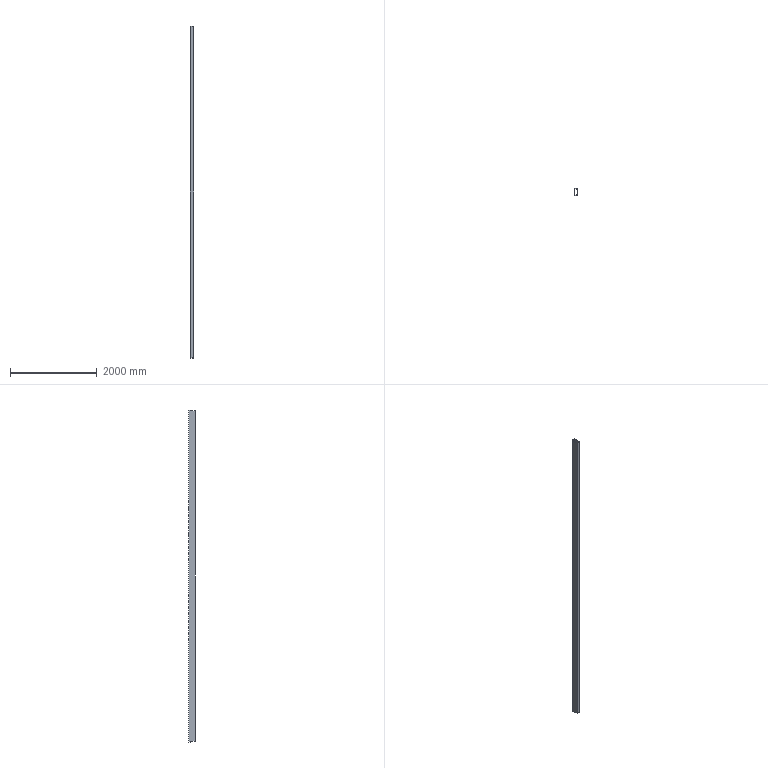Part | STEP file | 750078111 | 1 solid | 24 faces | box 80 x 160 x 7672 mm | volume 17309604 mm3 | plane 16 | cylinder 8 | commonest cylinder face diameters 4 x4 14 x4
STEP:
#1=CARTESIAN_POINT('',(-35.,-73.,3822.));
#2=VERTEX_POINT('',#1);
#3=CARTESIAN_POINT('',(-35.,28.5,3822.));
#4=VERTEX_POINT('',#3);
#5=CARTESIAN_POINT('',(-35.,-73.,3822.));
#6=DIRECTION('',(0.,1.,0.));
#7=VECTOR('',#6,1000.);
#8=LINE('',#5,#7);
#9=EDGE_CURVE('',#2,#4,#8,.T.);
#10=ORIENTED_EDGE('',*,*,#9,.F.);
#11=CARTESIAN_POINT('',(-35.,-73.,-3822.));
#12=VERTEX_POINT('',#11);
#13=CARTESIAN_POINT('',(-35.,-73.,3836.));
#14=DIRECTION('',(0.,0.,1.));
#15=VECTOR('',#14,1000.);
#16=LINE('',#13,#15);
#17=EDGE_CURVE('',#12,#2,#16,.T.);
#18=ORIENTED_EDGE('',*,*,#17,.F.);
#19=CARTESIAN_POINT('',(-35.,28.5,-3822.));
#20=VERTEX_POINT('',#19);
#21=CARTESIAN_POINT('',(-35.,-73.,-3822.));
#22=DIRECTION('',(0.,-1.,0.));
#23=VECTOR('',#22,1000.);
#24=LINE('',#21,#23);
#25=EDGE_CURVE('',#20,#12,#24,.T.);
#26=ORIENTED_EDGE('',*,*,#25,.F.);
#27=CARTESIAN_POINT('',(-35.,28.5,-3836.));
#28=VERTEX_POINT('',#27);
#29=CARTESIAN_POINT('',(-35.,28.5,3836.));
#30=DIRECTION('',(0.,0.,1.));
#31=VECTOR('',#30,1000.);
#32=LINE('',#29,#31);
#33=EDGE_CURVE('',#28,#20,#32,.T.);
#34=ORIENTED_EDGE('',*,*,#33,.F.);
#35=CARTESIAN_POINT('',(-35.,73.,-3836.));
#36=VERTEX_POINT('',#35);
#37=CARTESIAN_POINT('',(-35.,-73.,-3836.));
#38=DIRECTION('',(0.,-1.,0.));
#39=VECTOR('',#38,1000.);
#40=LINE('',#37,#39);
#41=EDGE_CURVE('',#36,#28,#40,.T.);
#42=ORIENTED_EDGE('',*,*,#41,.F.);
#43=CARTESIAN_POINT('',(-35.,73.,3836.));
#44=VERTEX_POINT('',#43);
#45=CARTESIAN_POINT('',(-35.,73.,3836.));
#46=DIRECTION('',(0.,0.,-1.));
#47=VECTOR('',#46,1000.);
#48=LINE('',#45,#47);
#49=EDGE_CURVE('',#44,#36,#48,.T.);
#50=ORIENTED_EDGE('',*,*,#49,.F.);
#51=CARTESIAN_POINT('',(-35.,28.5,3836.));
#52=VERTEX_POINT('',#51);
#53=CARTESIAN_POINT('',(-35.,-73.,3836.));
#54=DIRECTION('',(0.,1.,0.));
#55=VECTOR('',#54,1000.);
#56=LINE('',#53,#55);
#57=EDGE_CURVE('',#52,#44,#56,.T.);
#58=ORIENTED_EDGE('',*,*,#57,.F.);
#59=CARTESIAN_POINT('',(-35.,28.5,3836.));
#60=DIRECTION('',(0.,0.,1.));
#61=VECTOR('',#60,1000.);
#62=LINE('',#59,#61);
#63=EDGE_CURVE('',#4,#52,#62,.T.);
#64=ORIENTED_EDGE('',*,*,#63,.F.);
#65=EDGE_LOOP('',(#10,#18,#26,#34,#42,#50,#58,#64));
#66=FACE_OUTER_BOUND('',#65,.T.);
#67=CARTESIAN_POINT('',(-35.,-73.,3836.));
#68=DIRECTION('',(-1.,0.,0.));
#69=DIRECTION('',(0.,-1.,0.));
#70=AXIS2_PLACEMENT_3D('',#67,#68,#69);
#71=PLANE('',#70);
#72=ADVANCED_FACE('',(#66),#71,.F.);
#73=CARTESIAN_POINT('',(-40.,28.5,3822.));
#74=VERTEX_POINT('',#73);
#75=CARTESIAN_POINT('',(-40.,28.5,3836.));
#76=VERTEX_POINT('',#75);
#77=CARTESIAN_POINT('',(-40.,28.5,3822.));
#78=DIRECTION('',(0.,0.,1.));
#79=VECTOR('',#78,1000.);
#80=LINE('',#77,#79);
#81=EDGE_CURVE('',#74,#76,#80,.T.);
#82=ORIENTED_EDGE('',*,*,#81,.F.);
#83=CARTESIAN_POINT('',(-48.,28.5,3822.));
#84=DIRECTION('',(-1.,0.,0.));
#85=VECTOR('',#84,1000.);
#86=LINE('',#83,#85);
#87=EDGE_CURVE('',#4,#74,#86,.T.);
#88=ORIENTED_EDGE('',*,*,#87,.F.);
#89=ORIENTED_EDGE('',*,*,#63,.T.);
#90=CARTESIAN_POINT('',(-48.,28.5,3836.));
#91=DIRECTION('',(1.,0.,0.));
#92=VECTOR('',#91,1000.);
#93=LINE('',#90,#92);
#94=EDGE_CURVE('',#76,#52,#93,.T.);
#95=ORIENTED_EDGE('',*,*,#94,.F.);
#96=EDGE_LOOP('',(#82,#88,#89,#95));
#97=FACE_OUTER_BOUND('',#96,.T.);
#98=CARTESIAN_POINT('',(-48.,28.5,3822.));
#99=DIRECTION('',(0.,1.,0.));
#100=DIRECTION('',(-1.,0.,0.));
#101=AXIS2_PLACEMENT_3D('',#98,#99,#100);
#102=PLANE('',#101);
#103=ADVANCED_FACE('',(#97),#102,.F.);
#104=CARTESIAN_POINT('',(-40.,-73.,3822.));
#105=VERTEX_POINT('',#104);
#106=CARTESIAN_POINT('',(-40.,-80.,3822.));
#107=DIRECTION('',(0.,1.,0.));
#108=VECTOR('',#107,1000.);
#109=LINE('',#106,#108);
#110=EDGE_CURVE('',#105,#74,#109,.T.);
#111=ORIENTED_EDGE('',*,*,#110,.F.);
#112=CARTESIAN_POINT('',(-33.,-80.,3822.));
#113=VERTEX_POINT('',#112);
#114=CARTESIAN_POINT('',(-33.,-73.,3822.));
#115=DIRECTION('',(0.,0.,-1.));
#116=DIRECTION('',(-1.,0.,0.));
#117=AXIS2_PLACEMENT_3D('',#114,#115,#116);
#118=CIRCLE('',#117,7.);
#119=EDGE_CURVE('',#113,#105,#118,.T.);
#120=ORIENTED_EDGE('',*,*,#119,.F.);
#121=CARTESIAN_POINT('',(33.,-80.,3822.));
#122=VERTEX_POINT('',#121);
#123=CARTESIAN_POINT('',(-48.,-80.,3822.));
#124=DIRECTION('',(-1.,0.,0.));
#125=VECTOR('',#124,1000.);
#126=LINE('',#123,#125);
#127=EDGE_CURVE('',#122,#113,#126,.T.);
#128=ORIENTED_EDGE('',*,*,#127,.F.);
#129=CARTESIAN_POINT('',(40.,-73.,3822.));
#130=VERTEX_POINT('',#129);
#131=CARTESIAN_POINT('',(33.,-73.,3822.));
#132=DIRECTION('',(0.,0.,-1.));
#133=DIRECTION('',(-1.,0.,0.));
#134=AXIS2_PLACEMENT_3D('',#131,#132,#133);
#135=CIRCLE('',#134,7.);
#136=EDGE_CURVE('',#130,#122,#135,.T.);
#137=ORIENTED_EDGE('',*,*,#136,.F.);
#138=CARTESIAN_POINT('',(40.,28.5,3822.));
#139=VERTEX_POINT('',#138);
#140=CARTESIAN_POINT('',(40.,-80.,3822.));
#141=DIRECTION('',(0.,-1.,0.));
#142=VECTOR('',#141,1000.);
#143=LINE('',#140,#142);
#144=EDGE_CURVE('',#139,#130,#143,.T.);
#145=ORIENTED_EDGE('',*,*,#144,.F.);
#146=CARTESIAN_POINT('',(35.,28.5,3822.));
#147=VERTEX_POINT('',#146);
#148=CARTESIAN_POINT('',(-48.,28.5,3822.));
#149=DIRECTION('',(1.,0.,0.));
#150=VECTOR('',#149,1000.);
#151=LINE('',#148,#150);
#152=EDGE_CURVE('',#147,#139,#151,.T.);
#153=ORIENTED_EDGE('',*,*,#152,.F.);
#154=CARTESIAN_POINT('',(35.,-73.,3822.));
#155=VERTEX_POINT('',#154);
#156=CARTESIAN_POINT('',(35.,-80.,3822.));
#157=DIRECTION('',(0.,1.,0.));
#158=VECTOR('',#157,1000.);
#159=LINE('',#156,#158);
#160=EDGE_CURVE('',#155,#147,#159,.T.);
#161=ORIENTED_EDGE('',*,*,#160,.F.);
#162=CARTESIAN_POINT('',(33.,-75.,3822.));
#163=VERTEX_POINT('',#162);
#164=CARTESIAN_POINT('',(33.,-73.,3822.));
#165=DIRECTION('',(0.,0.,1.));
#166=DIRECTION('',(-1.,0.,0.));
#167=AXIS2_PLACEMENT_3D('',#164,#165,#166);
#168=CIRCLE('',#167,2.);
#169=EDGE_CURVE('',#163,#155,#168,.T.);
#170=ORIENTED_EDGE('',*,*,#169,.F.);
#171=CARTESIAN_POINT('',(-33.,-75.,3822.));
#172=VERTEX_POINT('',#171);
#173=CARTESIAN_POINT('',(-48.,-75.,3822.));
#174=DIRECTION('',(1.,0.,0.));
#175=VECTOR('',#174,1000.);
#176=LINE('',#173,#175);
#177=EDGE_CURVE('',#172,#163,#176,.T.);
#178=ORIENTED_EDGE('',*,*,#177,.F.);
#179=CARTESIAN_POINT('',(-33.,-73.,3822.));
#180=DIRECTION('',(0.,0.,1.));
#181=DIRECTION('',(-1.,0.,0.));
#182=AXIS2_PLACEMENT_3D('',#179,#180,#181);
#183=CIRCLE('',#182,2.);
#184=EDGE_CURVE('',#2,#172,#183,.T.);
#185=ORIENTED_EDGE('',*,*,#184,.F.);
#186=ORIENTED_EDGE('',*,*,#9,.T.);
#187=ORIENTED_EDGE('',*,*,#87,.T.);
#188=EDGE_LOOP('',(#111,#120,#128,#137,#145,#153,#161,#170,#178,#185,#186,#187));
#189=FACE_OUTER_BOUND('',#188,.T.);
#190=CARTESIAN_POINT('',(-48.,-80.,3822.));
#191=DIRECTION('',(0.,0.,-1.));
#192=DIRECTION('',(-1.,0.,0.));
#193=AXIS2_PLACEMENT_3D('',#190,#191,#192);
#194=PLANE('',#193);
#195=ADVANCED_FACE('',(#189),#194,.F.);
#196=ORIENTED_EDGE('',*,*,#184,.T.);
#197=CARTESIAN_POINT('',(-33.,-75.,-3822.));
#198=VERTEX_POINT('',#197);
#199=CARTESIAN_POINT('',(-33.,-75.,3836.));
#200=DIRECTION('',(0.,0.,1.));
#201=VECTOR('',#200,1000.);
#202=LINE('',#199,#201);
#203=EDGE_CURVE('',#198,#172,#202,.T.);
#204=ORIENTED_EDGE('',*,*,#203,.F.);
#205=CARTESIAN_POINT('',(-33.,-73.,-3822.));
#206=DIRECTION('',(0.,0.,1.));
#207=DIRECTION('',(-1.,0.,0.));
#208=AXIS2_PLACEMENT_3D('',#205,#206,#207);
#209=CIRCLE('',#208,2.);
#210=EDGE_CURVE('',#12,#198,#209,.T.);
#211=ORIENTED_EDGE('',*,*,#210,.F.);
#212=ORIENTED_EDGE('',*,*,#17,.T.);
#213=EDGE_LOOP('',(#196,#204,#211,#212));
#214=FACE_OUTER_BOUND('',#213,.T.);
#215=CARTESIAN_POINT('',(-33.,-73.,3836.));
#216=DIRECTION('',(0.,0.,-1.));
#217=DIRECTION('',(-1.,0.,0.));
#218=AXIS2_PLACEMENT_3D('',#215,#216,#217);
#219=CYLINDRICAL_SURFACE('',#218,2.);
#220=ADVANCED_FACE('',(#214),#219,.F.);
#221=CARTESIAN_POINT('',(33.,-75.,-3822.));
#222=VERTEX_POINT('',#221);
#223=CARTESIAN_POINT('',(-48.,-75.,-3822.));
#224=DIRECTION('',(-1.,0.,0.));
#225=VECTOR('',#224,1000.);
#226=LINE('',#223,#225);
#227=EDGE_CURVE('',#222,#198,#226,.T.);
#228=ORIENTED_EDGE('',*,*,#227,.F.);
#229=CARTESIAN_POINT('',(35.,-73.,-3822.));
#230=VERTEX_POINT('',#229);
#231=CARTESIAN_POINT('',(33.,-73.,-3822.));
#232=DIRECTION('',(0.,0.,-1.));
#233=DIRECTION('',(-1.,0.,0.));
#234=AXIS2_PLACEMENT_3D('',#231,#232,#233);
#235=CIRCLE('',#234,2.);
#236=EDGE_CURVE('',#230,#222,#235,.T.);
#237=ORIENTED_EDGE('',*,*,#236,.F.);
#238=CARTESIAN_POINT('',(35.,28.5,-3822.));
#239=VERTEX_POINT('',#238);
#240=CARTESIAN_POINT('',(35.,28.5,-3822.));
#241=DIRECTION('',(0.,-1.,0.));
#242=VECTOR('',#241,1000.);
#243=LINE('',#240,#242);
#244=EDGE_CURVE('',#239,#230,#243,.T.);
#245=ORIENTED_EDGE('',*,*,#244,.F.);
#246=CARTESIAN_POINT('',(40.,28.5,-3822.));
#247=VERTEX_POINT('',#246);
#248=CARTESIAN_POINT('',(-48.,28.5,-3822.));
#249=DIRECTION('',(-1.,0.,0.));
#250=VECTOR('',#249,1000.);
#251=LINE('',#248,#250);
#252=EDGE_CURVE('',#247,#239,#251,.T.);
#253=ORIENTED_EDGE('',*,*,#252,.F.);
#254=CARTESIAN_POINT('',(40.,-73.,-3822.));
#255=VERTEX_POINT('',#254);
#256=CARTESIAN_POINT('',(40.,28.5,-3822.));
#257=DIRECTION('',(0.,1.,0.));
#258=VECTOR('',#257,1000.);
#259=LINE('',#256,#258);
#260=EDGE_CURVE('',#255,#247,#259,.T.);
#261=ORIENTED_EDGE('',*,*,#260,.F.);
#262=CARTESIAN_POINT('',(33.,-80.,-3822.));
#263=VERTEX_POINT('',#262);
#264=CARTESIAN_POINT('',(33.,-73.,-3822.));
#265=DIRECTION('',(0.,0.,1.));
#266=DIRECTION('',(-1.,0.,0.));
#267=AXIS2_PLACEMENT_3D('',#264,#265,#266);
#268=CIRCLE('',#267,7.);
#269=EDGE_CURVE('',#263,#255,#268,.T.);
#270=ORIENTED_EDGE('',*,*,#269,.F.);
#271=CARTESIAN_POINT('',(-33.,-80.,-3822.));
#272=VERTEX_POINT('',#271);
#273=CARTESIAN_POINT('',(-48.,-80.,-3822.));
#274=DIRECTION('',(1.,0.,0.));
#275=VECTOR('',#274,1000.);
#276=LINE('',#273,#275);
#277=EDGE_CURVE('',#272,#263,#276,.T.);
#278=ORIENTED_EDGE('',*,*,#277,.F.);
#279=CARTESIAN_POINT('',(-40.,-73.,-3822.));
#280=VERTEX_POINT('',#279);
#281=CARTESIAN_POINT('',(-33.,-73.,-3822.));
#282=DIRECTION('',(0.,0.,1.));
#283=DIRECTION('',(-1.,0.,0.));
#284=AXIS2_PLACEMENT_3D('',#281,#282,#283);
#285=CIRCLE('',#284,7.);
#286=EDGE_CURVE('',#280,#272,#285,.T.);
#287=ORIENTED_EDGE('',*,*,#286,.F.);
#288=CARTESIAN_POINT('',(-40.,28.5,-3822.));
#289=VERTEX_POINT('',#288);
#290=CARTESIAN_POINT('',(-40.,28.5,-3822.));
#291=DIRECTION('',(0.,-1.,0.));
#292=VECTOR('',#291,1000.);
#293=LINE('',#290,#292);
#294=EDGE_CURVE('',#289,#280,#293,.T.);
#295=ORIENTED_EDGE('',*,*,#294,.F.);
#296=CARTESIAN_POINT('',(-48.,28.5,-3822.));
#297=DIRECTION('',(-1.,0.,0.));
#298=VECTOR('',#297,1000.);
#299=LINE('',#296,#298);
#300=EDGE_CURVE('',#20,#289,#299,.T.);
#301=ORIENTED_EDGE('',*,*,#300,.F.);
#302=ORIENTED_EDGE('',*,*,#25,.T.);
#303=ORIENTED_EDGE('',*,*,#210,.T.);
#304=EDGE_LOOP('',(#228,#237,#245,#253,#261,#270,#278,#287,#295,#301,#302,#303));
#305=FACE_OUTER_BOUND('',#304,.T.);
#306=CARTESIAN_POINT('',(-48.,28.5,-3822.));
#307=DIRECTION('',(0.,0.,1.));
#308=DIRECTION('',(1.,0.,0.));
#309=AXIS2_PLACEMENT_3D('',#306,#307,#308);
#310=PLANE('',#309);
#311=ADVANCED_FACE('',(#305),#310,.F.);
#312=CARTESIAN_POINT('',(-40.,28.5,-3836.));
#313=VERTEX_POINT('',#312);
#314=CARTESIAN_POINT('',(-40.,28.5,-3836.));
#315=DIRECTION('',(0.,0.,1.));
#316=VECTOR('',#315,1000.);
#317=LINE('',#314,#316);
#318=EDGE_CURVE('',#313,#289,#317,.T.);
#319=ORIENTED_EDGE('',*,*,#318,.F.);
#320=CARTESIAN_POINT('',(-48.,28.5,-3836.));
#321=DIRECTION('',(-1.,0.,0.));
#322=VECTOR('',#321,1000.);
#323=LINE('',#320,#322);
#324=EDGE_CURVE('',#28,#313,#323,.T.);
#325=ORIENTED_EDGE('',*,*,#324,.F.);
#326=ORIENTED_EDGE('',*,*,#33,.T.);
#327=ORIENTED_EDGE('',*,*,#300,.T.);
#328=EDGE_LOOP('',(#319,#325,#326,#327));
#329=FACE_OUTER_BOUND('',#328,.T.);
#330=CARTESIAN_POINT('',(-48.,28.5,-3836.));
#331=DIRECTION('',(0.,1.,0.));
#332=DIRECTION('',(-1.,0.,0.));
#333=AXIS2_PLACEMENT_3D('',#330,#331,#332);
#334=PLANE('',#333);
#335=ADVANCED_FACE('',(#329),#334,.F.);
#336=CARTESIAN_POINT('',(-33.,75.,-3836.));
#337=VERTEX_POINT('',#336);
#338=CARTESIAN_POINT('',(-33.,73.,-3836.));
#339=DIRECTION('',(0.,0.,1.));
#340=DIRECTION('',(-1.,0.,0.));
#341=AXIS2_PLACEMENT_3D('',#338,#339,#340);
#342=CIRCLE('',#341,2.);
#343=EDGE_CURVE('',#337,#36,#342,.T.);
#344=ORIENTED_EDGE('',*,*,#343,.T.);
#345=ORIENTED_EDGE('',*,*,#41,.T.);
#346=ORIENTED_EDGE('',*,*,#324,.T.);
#347=CARTESIAN_POINT('',(-40.,73.,-3836.));
#348=VERTEX_POINT('',#347);
#349=CARTESIAN_POINT('',(-40.,-73.,-3836.));
#350=DIRECTION('',(0.,1.,0.));
#351=VECTOR('',#350,1000.);
#352=LINE('',#349,#351);
#353=EDGE_CURVE('',#313,#348,#352,.T.);
#354=ORIENTED_EDGE('',*,*,#353,.T.);
#355=CARTESIAN_POINT('',(-33.,80.,-3836.));
#356=VERTEX_POINT('',#355);
#357=CARTESIAN_POINT('',(-33.,73.,-3836.));
#358=DIRECTION('',(0.,0.,-1.));
#359=DIRECTION('',(-1.,0.,0.));
#360=AXIS2_PLACEMENT_3D('',#357,#358,#359);
#361=CIRCLE('',#360,7.);
#362=EDGE_CURVE('',#348,#356,#361,.T.);
#363=ORIENTED_EDGE('',*,*,#362,.T.);
#364=CARTESIAN_POINT('',(33.,80.,-3836.));
#365=VERTEX_POINT('',#364);
#366=CARTESIAN_POINT('',(33.,80.,-3836.));
#367=DIRECTION('',(1.,0.,0.));
#368=VECTOR('',#367,1000.);
#369=LINE('',#366,#368);
#370=EDGE_CURVE('',#356,#365,#369,.T.);
#371=ORIENTED_EDGE('',*,*,#370,.T.);
#372=CARTESIAN_POINT('',(40.,73.,-3836.));
#373=VERTEX_POINT('',#372);
#374=CARTESIAN_POINT('',(33.,73.,-3836.));
#375=DIRECTION('',(0.,0.,-1.));
#376=DIRECTION('',(-1.,0.,0.));
#377=AXIS2_PLACEMENT_3D('',#374,#375,#376);
#378=CIRCLE('',#377,7.);
#379=EDGE_CURVE('',#365,#373,#378,.T.);
#380=ORIENTED_EDGE('',*,*,#379,.T.);
#381=CARTESIAN_POINT('',(40.,28.5,-3836.));
#382=VERTEX_POINT('',#381);
#383=CARTESIAN_POINT('',(40.,-73.,-3836.));
#384=DIRECTION('',(0.,-1.,0.));
#385=VECTOR('',#384,1000.);
#386=LINE('',#383,#385);
#387=EDGE_CURVE('',#373,#382,#386,.T.);
#388=ORIENTED_EDGE('',*,*,#387,.T.);
#389=CARTESIAN_POINT('',(35.,28.5,-3836.));
#390=VERTEX_POINT('',#389);
#391=CARTESIAN_POINT('',(33.,28.5,-3836.));
#392=DIRECTION('',(-1.,0.,0.));
#393=VECTOR('',#392,1000.);
#394=LINE('',#391,#393);
#395=EDGE_CURVE('',#382,#390,#394,.T.);
#396=ORIENTED_EDGE('',*,*,#395,.T.);
#397=CARTESIAN_POINT('',(35.,73.,-3836.));
#398=VERTEX_POINT('',#397);
#399=CARTESIAN_POINT('',(35.,-73.,-3836.));
#400=DIRECTION('',(0.,1.,0.));
#401=VECTOR('',#400,1000.);
#402=LINE('',#399,#401);
#403=EDGE_CURVE('',#390,#398,#402,.T.);
#404=ORIENTED_EDGE('',*,*,#403,.T.);
#405=CARTESIAN_POINT('',(33.,75.,-3836.));
#406=VERTEX_POINT('',#405);
#407=CARTESIAN_POINT('',(33.,73.,-3836.));
#408=DIRECTION('',(0.,0.,1.));
#409=DIRECTION('',(-1.,0.,0.));
#410=AXIS2_PLACEMENT_3D('',#407,#408,#409);
#411=CIRCLE('',#410,2.);
#412=EDGE_CURVE('',#398,#406,#411,.T.);
#413=ORIENTED_EDGE('',*,*,#412,.T.);
#414=CARTESIAN_POINT('',(33.,75.,-3836.));
#415=DIRECTION('',(-1.,0.,0.));
#416=VECTOR('',#415,1000.);
#417=LINE('',#414,#416);
#418=EDGE_CURVE('',#406,#337,#417,.T.);
#419=ORIENTED_EDGE('',*,*,#418,.T.);
#420=EDGE_LOOP('',(#344,#345,#346,#354,#363,#371,#380,#388,#396,#404,#413,#419));
#421=FACE_OUTER_BOUND('',#420,.T.);
#422=CARTESIAN_POINT('',(33.,-73.,-3836.));
#423=DIRECTION('',(0.,0.,-1.));
#424=DIRECTION('',(-1.,0.,0.));
#425=AXIS2_PLACEMENT_3D('',#422,#423,#424);
#426=PLANE('',#425);
#427=ADVANCED_FACE('',(#421),#426,.T.);
#428=CARTESIAN_POINT('',(-33.,75.,3836.));
#429=VERTEX_POINT('',#428);
#430=CARTESIAN_POINT('',(-33.,75.,3836.));
#431=DIRECTION('',(0.,0.,-1.));
#432=VECTOR('',#431,1000.);
#433=LINE('',#430,#432);
#434=EDGE_CURVE('',#429,#337,#433,.T.);
#435=ORIENTED_EDGE('',*,*,#434,.F.);
#436=CARTESIAN_POINT('',(-33.,73.,3836.));
#437=DIRECTION('',(0.,0.,-1.));
#438=DIRECTION('',(-1.,0.,0.));
#439=AXIS2_PLACEMENT_3D('',#436,#437,#438);
#440=CIRCLE('',#439,2.);
#441=EDGE_CURVE('',#44,#429,#440,.T.);
#442=ORIENTED_EDGE('',*,*,#441,.F.);
#443=ORIENTED_EDGE('',*,*,#49,.T.);
#444=ORIENTED_EDGE('',*,*,#343,.F.);
#445=EDGE_LOOP('',(#435,#442,#443,#444));
#446=FACE_OUTER_BOUND('',#445,.T.);
#447=CARTESIAN_POINT('',(-33.,73.,3836.));
#448=DIRECTION('',(0.,0.,-1.));
#449=DIRECTION('',(-1.,0.,0.));
#450=AXIS2_PLACEMENT_3D('',#447,#448,#449);
#451=CYLINDRICAL_SURFACE('',#450,2.);
#452=ADVANCED_FACE('',(#446),#451,.F.);
#453=ORIENTED_EDGE('',*,*,#94,.T.);
#454=ORIENTED_EDGE('',*,*,#57,.T.);
#455=ORIENTED_EDGE('',*,*,#441,.T.);
#456=CARTESIAN_POINT('',(33.,75.,3836.));
#457=VERTEX_POINT('',#456);
#458=CARTESIAN_POINT('',(33.,75.,3836.));
#459=DIRECTION('',(-1.,0.,0.));
#460=VECTOR('',#459,1000.);
#461=LINE('',#458,#460);
#462=EDGE_CURVE('',#457,#429,#461,.T.);
#463=ORIENTED_EDGE('',*,*,#462,.F.);
#464=CARTESIAN_POINT('',(35.,73.,3836.));
#465=VERTEX_POINT('',#464);
#466=CARTESIAN_POINT('',(33.,73.,3836.));
#467=DIRECTION('',(0.,0.,1.));
#468=DIRECTION('',(-1.,0.,0.));
#469=AXIS2_PLACEMENT_3D('',#466,#467,#468);
#470=CIRCLE('',#469,2.);
#471=EDGE_CURVE('',#465,#457,#470,.T.);
#472=ORIENTED_EDGE('',*,*,#471,.F.);
#473=CARTESIAN_POINT('',(35.,28.5,3836.));
#474=VERTEX_POINT('',#473);
#475=CARTESIAN_POINT('',(35.,-73.,3836.));
#476=DIRECTION('',(0.,1.,0.));
#477=VECTOR('',#476,1000.);
#478=LINE('',#475,#477);
#479=EDGE_CURVE('',#474,#465,#478,.T.);
#480=ORIENTED_EDGE('',*,*,#479,.F.);
#481=CARTESIAN_POINT('',(40.,28.5,3836.));
#482=VERTEX_POINT('',#481);
#483=CARTESIAN_POINT('',(33.,28.5,3836.));
#484=DIRECTION('',(-1.,0.,0.));
#485=VECTOR('',#484,1000.);
#486=LINE('',#483,#485);
#487=EDGE_CURVE('',#482,#474,#486,.T.);
#488=ORIENTED_EDGE('',*,*,#487,.F.);
#489=CARTESIAN_POINT('',(40.,73.,3836.));
#490=VERTEX_POINT('',#489);
#491=CARTESIAN_POINT('',(40.,-73.,3836.));
#492=DIRECTION('',(0.,-1.,0.));
#493=VECTOR('',#492,1000.);
#494=LINE('',#491,#493);
#495=EDGE_CURVE('',#490,#482,#494,.T.);
#496=ORIENTED_EDGE('',*,*,#495,.F.);
#497=CARTESIAN_POINT('',(33.,80.,3836.));
#498=VERTEX_POINT('',#497);
#499=CARTESIAN_POINT('',(33.,73.,3836.));
#500=DIRECTION('',(0.,0.,-1.));
#501=DIRECTION('',(-1.,0.,0.));
#502=AXIS2_PLACEMENT_3D('',#499,#500,#501);
#503=CIRCLE('',#502,7.);
#504=EDGE_CURVE('',#498,#490,#503,.T.);
#505=ORIENTED_EDGE('',*,*,#504,.F.);
#506=CARTESIAN_POINT('',(-33.,80.,3836.));
#507=VERTEX_POINT('',#506);
#508=CARTESIAN_POINT('',(33.,80.,3836.));
#509=DIRECTION('',(1.,0.,0.));
#510=VECTOR('',#509,1000.);
#511=LINE('',#508,#510);
#512=EDGE_CURVE('',#507,#498,#511,.T.);
#513=ORIENTED_EDGE('',*,*,#512,.F.);
#514=CARTESIAN_POINT('',(-40.,73.,3836.));
#515=VERTEX_POINT('',#514);
#516=CARTESIAN_POINT('',(-33.,73.,3836.));
#517=DIRECTION('',(0.,0.,-1.));
#518=DIRECTION('',(-1.,0.,0.));
#519=AXIS2_PLACEMENT_3D('',#516,#517,#518);
#520=CIRCLE('',#519,7.);
#521=EDGE_CURVE('',#515,#507,#520,.T.);
#522=ORIENTED_EDGE('',*,*,#521,.F.);
#523=CARTESIAN_POINT('',(-40.,-73.,3836.));
#524=DIRECTION('',(0.,1.,0.));
#525=VECTOR('',#524,1000.);
#526=LINE('',#523,#525);
#527=EDGE_CURVE('',#76,#515,#526,.T.);
#528=ORIENTED_EDGE('',*,*,#527,.F.);
#529=EDGE_LOOP('',(#453,#454,#455,#463,#472,#480,#488,#496,#505,#513,#522,#528));
#530=FACE_OUTER_BOUND('',#529,.T.);
#531=CARTESIAN_POINT('',(33.,-73.,3836.));
#532=DIRECTION('',(0.,0.,-1.));
#533=DIRECTION('',(-1.,0.,0.));
#534=AXIS2_PLACEMENT_3D('',#531,#532,#533);
#535=PLANE('',#534);
#536=ADVANCED_FACE('',(#530),#535,.F.);
#537=ORIENTED_EDGE('',*,*,#294,.T.);
#538=CARTESIAN_POINT('',(-40.,-73.,3836.));
#539=DIRECTION('',(0.,0.,1.));
#540=VECTOR('',#539,1000.);
#541=LINE('',#538,#540);
#542=EDGE_CURVE('',#280,#105,#541,.T.);
#543=ORIENTED_EDGE('',*,*,#542,.T.);
#544=ORIENTED_EDGE('',*,*,#110,.T.);
#545=ORIENTED_EDGE('',*,*,#81,.T.);
#546=ORIENTED_EDGE('',*,*,#527,.T.);
#547=CARTESIAN_POINT('',(-40.,73.,3836.));
#548=DIRECTION('',(0.,0.,-1.));
#549=VECTOR('',#548,1000.);
#550=LINE('',#547,#549);
#551=EDGE_CURVE('',#515,#348,#550,.T.);
#552=ORIENTED_EDGE('',*,*,#551,.T.);
#553=ORIENTED_EDGE('',*,*,#353,.F.);
#554=ORIENTED_EDGE('',*,*,#318,.T.);
#555=EDGE_LOOP('',(#537,#543,#544,#545,#546,#552,#553,#554));
#556=FACE_OUTER_BOUND('',#555,.T.);
#557=CARTESIAN_POINT('',(-40.,-73.,3836.));
#558=DIRECTION('',(-1.,0.,0.));
#559=DIRECTION('',(0.,0.,1.));
#560=AXIS2_PLACEMENT_3D('',#557,#558,#559);
#561=PLANE('',#560);
#562=ADVANCED_FACE('',(#556),#561,.T.);
#563=ORIENTED_EDGE('',*,*,#286,.T.);
#564=CARTESIAN_POINT('',(-33.,-80.,3836.));
#565=DIRECTION('',(0.,0.,1.));
#566=VECTOR('',#565,1000.);
#567=LINE('',#564,#566);
#568=EDGE_CURVE('',#272,#113,#567,.T.);
#569=ORIENTED_EDGE('',*,*,#568,.T.);
#570=ORIENTED_EDGE('',*,*,#119,.T.);
#571=ORIENTED_EDGE('',*,*,#542,.F.);
#572=EDGE_LOOP('',(#563,#569,#570,#571));
#573=FACE_OUTER_BOUND('',#572,.T.);
#574=CARTESIAN_POINT('',(-33.,-73.,3836.));
#575=DIRECTION('',(0.,0.,-1.));
#576=DIRECTION('',(-1.,0.,0.));
#577=AXIS2_PLACEMENT_3D('',#574,#575,#576);
#578=CYLINDRICAL_SURFACE('',#577,7.);
#579=ADVANCED_FACE('',(#573),#578,.T.);
#580=ORIENTED_EDGE('',*,*,#277,.T.);
#581=CARTESIAN_POINT('',(33.,-80.,3836.));
#582=DIRECTION('',(0.,0.,1.));
#583=VECTOR('',#582,1000.);
#584=LINE('',#581,#583);
#585=EDGE_CURVE('',#263,#122,#584,.T.);
#586=ORIENTED_EDGE('',*,*,#585,.T.);
#587=ORIENTED_EDGE('',*,*,#127,.T.);
#588=ORIENTED_EDGE('',*,*,#568,.F.);
#589=EDGE_LOOP('',(#580,#586,#587,#588));
#590=FACE_OUTER_BOUND('',#589,.T.);
#591=CARTESIAN_POINT('',(33.,-80.,3836.));
#592=DIRECTION('',(0.,-1.,0.));
#593=DIRECTION('',(0.,0.,-1.));
#594=AXIS2_PLACEMENT_3D('',#591,#592,#593);
#595=PLANE('',#594);
#596=ADVANCED_FACE('',(#590),#595,.T.);
#597=ORIENTED_EDGE('',*,*,#269,.T.);
#598=CARTESIAN_POINT('',(40.,-73.,3836.));
#599=DIRECTION('',(0.,0.,1.));
#600=VECTOR('',#599,1000.);
#601=LINE('',#598,#600);
#602=EDGE_CURVE('',#255,#130,#601,.T.);
#603=ORIENTED_EDGE('',*,*,#602,.T.);
#604=ORIENTED_EDGE('',*,*,#136,.T.);
#605=ORIENTED_EDGE('',*,*,#585,.F.);
#606=EDGE_LOOP('',(#597,#603,#604,#605));
#607=FACE_OUTER_BOUND('',#606,.T.);
#608=CARTESIAN_POINT('',(33.,-73.,3836.));
#609=DIRECTION('',(0.,0.,-1.));
#610=DIRECTION('',(-1.,0.,0.));
#611=AXIS2_PLACEMENT_3D('',#608,#609,#610);
#612=CYLINDRICAL_SURFACE('',#611,7.);
#613=ADVANCED_FACE('',(#607),#612,.T.);
#614=ORIENTED_EDGE('',*,*,#495,.T.);
#615=CARTESIAN_POINT('',(40.,28.5,3836.));
#616=DIRECTION('',(0.,0.,-1.));
#617=VECTOR('',#616,1000.);
#618=LINE('',#615,#617);
#619=EDGE_CURVE('',#482,#139,#618,.T.);
#620=ORIENTED_EDGE('',*,*,#619,.T.);
#621=ORIENTED_EDGE('',*,*,#144,.T.);
#622=ORIENTED_EDGE('',*,*,#602,.F.);
#623=ORIENTED_EDGE('',*,*,#260,.T.);
#624=CARTESIAN_POINT('',(40.,28.5,3836.));
#625=DIRECTION('',(0.,0.,-1.));
#626=VECTOR('',#625,1000.);
#627=LINE('',#624,#626);
#628=EDGE_CURVE('',#247,#382,#627,.T.);
#629=ORIENTED_EDGE('',*,*,#628,.T.);
#630=ORIENTED_EDGE('',*,*,#387,.F.);
#631=CARTESIAN_POINT('',(40.,73.,3836.));
#632=DIRECTION('',(0.,0.,1.));
#633=VECTOR('',#632,1000.);
#634=LINE('',#631,#633);
#635=EDGE_CURVE('',#373,#490,#634,.T.);
#636=ORIENTED_EDGE('',*,*,#635,.T.);
#637=EDGE_LOOP('',(#614,#620,#621,#622,#623,#629,#630,#636));
#638=FACE_OUTER_BOUND('',#637,.T.);
#639=CARTESIAN_POINT('',(40.,73.,3836.));
#640=DIRECTION('',(1.,0.,0.));
#641=DIRECTION('',(0.,1.,0.));
#642=AXIS2_PLACEMENT_3D('',#639,#640,#641);
#643=PLANE('',#642);
#644=ADVANCED_FACE('',(#638),#643,.T.);
#645=ORIENTED_EDGE('',*,*,#619,.F.);
#646=ORIENTED_EDGE('',*,*,#487,.T.);
#647=CARTESIAN_POINT('',(35.,28.5,3822.));
#648=DIRECTION('',(0.,0.,1.));
#649=VECTOR('',#648,1000.);
#650=LINE('',#647,#649);
#651=EDGE_CURVE('',#147,#474,#650,.T.);
#652=ORIENTED_EDGE('',*,*,#651,.F.);
#653=ORIENTED_EDGE('',*,*,#152,.T.);
#654=EDGE_LOOP('',(#645,#646,#652,#653));
#655=FACE_OUTER_BOUND('',#654,.T.);
#656=CARTESIAN_POINT('',(-48.,28.5,3822.));
#657=DIRECTION('',(0.,1.,0.));
#658=DIRECTION('',(-1.,0.,0.));
#659=AXIS2_PLACEMENT_3D('',#656,#657,#658);
#660=PLANE('',#659);
#661=ADVANCED_FACE('',(#655),#660,.F.);
#662=ORIENTED_EDGE('',*,*,#160,.T.);
#663=ORIENTED_EDGE('',*,*,#651,.T.);
#664=ORIENTED_EDGE('',*,*,#479,.T.);
#665=CARTESIAN_POINT('',(35.,73.,3836.));
#666=DIRECTION('',(0.,0.,1.));
#667=VECTOR('',#666,1000.);
#668=LINE('',#665,#667);
#669=EDGE_CURVE('',#398,#465,#668,.T.);
#670=ORIENTED_EDGE('',*,*,#669,.F.);
#671=ORIENTED_EDGE('',*,*,#403,.F.);
#672=CARTESIAN_POINT('',(35.,28.5,3836.));
#673=DIRECTION('',(0.,0.,-1.));
#674=VECTOR('',#673,1000.);
#675=LINE('',#672,#674);
#676=EDGE_CURVE('',#239,#390,#675,.T.);
#677=ORIENTED_EDGE('',*,*,#676,.F.);
#678=ORIENTED_EDGE('',*,*,#244,.T.);
#679=CARTESIAN_POINT('',(35.,-73.,3836.));
#680=DIRECTION('',(0.,0.,-1.));
#681=VECTOR('',#680,1000.);
#682=LINE('',#679,#681);
#683=EDGE_CURVE('',#155,#230,#682,.T.);
#684=ORIENTED_EDGE('',*,*,#683,.F.);
#685=EDGE_LOOP('',(#662,#663,#664,#670,#671,#677,#678,#684));
#686=FACE_OUTER_BOUND('',#685,.T.);
#687=CARTESIAN_POINT('',(35.,73.,3836.));
#688=DIRECTION('',(1.,0.,0.));
#689=DIRECTION('',(0.,1.,0.));
#690=AXIS2_PLACEMENT_3D('',#687,#688,#689);
#691=PLANE('',#690);
#692=ADVANCED_FACE('',(#686),#691,.F.);
#693=ORIENTED_EDGE('',*,*,#169,.T.);
#694=ORIENTED_EDGE('',*,*,#683,.T.);
#695=ORIENTED_EDGE('',*,*,#236,.T.);
#696=CARTESIAN_POINT('',(33.,-75.,3836.));
#697=DIRECTION('',(0.,0.,-1.));
#698=VECTOR('',#697,1000.);
#699=LINE('',#696,#698);
#700=EDGE_CURVE('',#163,#222,#699,.T.);
#701=ORIENTED_EDGE('',*,*,#700,.F.);
#702=EDGE_LOOP('',(#693,#694,#695,#701));
#703=FACE_OUTER_BOUND('',#702,.T.);
#704=CARTESIAN_POINT('',(33.,-73.,3836.));
#705=DIRECTION('',(0.,0.,-1.));
#706=DIRECTION('',(-1.,0.,0.));
#707=AXIS2_PLACEMENT_3D('',#704,#705,#706);
#708=CYLINDRICAL_SURFACE('',#707,2.);
#709=ADVANCED_FACE('',(#703),#708,.F.);
#710=ORIENTED_EDGE('',*,*,#177,.T.);
#711=ORIENTED_EDGE('',*,*,#700,.T.);
#712=ORIENTED_EDGE('',*,*,#227,.T.);
#713=ORIENTED_EDGE('',*,*,#203,.T.);
#714=EDGE_LOOP('',(#710,#711,#712,#713));
#715=FACE_OUTER_BOUND('',#714,.T.);
#716=CARTESIAN_POINT('',(33.,-75.,3836.));
#717=DIRECTION('',(0.,-1.,0.));
#718=DIRECTION('',(0.,0.,-1.));
#719=AXIS2_PLACEMENT_3D('',#716,#717,#718);
#720=PLANE('',#719);
#721=ADVANCED_FACE('',(#715),#720,.F.);
#722=ORIENTED_EDGE('',*,*,#628,.F.);
#723=ORIENTED_EDGE('',*,*,#252,.T.);
#724=ORIENTED_EDGE('',*,*,#676,.T.);
#725=ORIENTED_EDGE('',*,*,#395,.F.);
#726=EDGE_LOOP('',(#722,#723,#724,#725));
#727=FACE_OUTER_BOUND('',#726,.T.);
#728=CARTESIAN_POINT('',(-48.,28.5,-3836.));
#729=DIRECTION('',(0.,1.,0.));
#730=DIRECTION('',(-1.,0.,0.));
#731=AXIS2_PLACEMENT_3D('',#728,#729,#730);
#732=PLANE('',#731);
#733=ADVANCED_FACE('',(#727),#732,.F.);
#734=CARTESIAN_POINT('',(33.,75.,3836.));
#735=DIRECTION('',(0.,0.,-1.));
#736=VECTOR('',#735,1000.);
#737=LINE('',#734,#736);
#738=EDGE_CURVE('',#457,#406,#737,.T.);
#739=ORIENTED_EDGE('',*,*,#738,.F.);
#740=ORIENTED_EDGE('',*,*,#462,.T.);
#741=ORIENTED_EDGE('',*,*,#434,.T.);
#742=ORIENTED_EDGE('',*,*,#418,.F.);
#743=EDGE_LOOP('',(#739,#740,#741,#742));
#744=FACE_OUTER_BOUND('',#743,.T.);
#745=CARTESIAN_POINT('',(-33.,75.,3836.));
#746=DIRECTION('',(0.,1.,0.));
#747=DIRECTION('',(0.,0.,1.));
#748=AXIS2_PLACEMENT_3D('',#745,#746,#747);
#749=PLANE('',#748);
#750=ADVANCED_FACE('',(#744),#749,.F.);
#751=ORIENTED_EDGE('',*,*,#669,.T.);
#752=ORIENTED_EDGE('',*,*,#471,.T.);
#753=ORIENTED_EDGE('',*,*,#738,.T.);
#754=ORIENTED_EDGE('',*,*,#412,.F.);
#755=EDGE_LOOP('',(#751,#752,#753,#754));
#756=FACE_OUTER_BOUND('',#755,.T.);
#757=CARTESIAN_POINT('',(33.,73.,3836.));
#758=DIRECTION('',(0.,0.,-1.));
#759=DIRECTION('',(-1.,0.,0.));
#760=AXIS2_PLACEMENT_3D('',#757,#758,#759);
#761=CYLINDRICAL_SURFACE('',#760,2.);
#762=ADVANCED_FACE('',(#756),#761,.F.);
#763=ORIENTED_EDGE('',*,*,#504,.T.);
#764=ORIENTED_EDGE('',*,*,#635,.F.);
#765=ORIENTED_EDGE('',*,*,#379,.F.);
#766=CARTESIAN_POINT('',(33.,80.,3836.));
#767=DIRECTION('',(0.,0.,1.));
#768=VECTOR('',#767,1000.);
#769=LINE('',#766,#768);
#770=EDGE_CURVE('',#365,#498,#769,.T.);
#771=ORIENTED_EDGE('',*,*,#770,.T.);
#772=EDGE_LOOP('',(#763,#764,#765,#771));
#773=FACE_OUTER_BOUND('',#772,.T.);
#774=CARTESIAN_POINT('',(33.,73.,3836.));
#775=DIRECTION('',(0.,0.,-1.));
#776=DIRECTION('',(-1.,0.,0.));
#777=AXIS2_PLACEMENT_3D('',#774,#775,#776);
#778=CYLINDRICAL_SURFACE('',#777,7.);
#779=ADVANCED_FACE('',(#773),#778,.T.);
#780=ORIENTED_EDGE('',*,*,#512,.T.);
#781=ORIENTED_EDGE('',*,*,#770,.F.);
#782=ORIENTED_EDGE('',*,*,#370,.F.);
#783=CARTESIAN_POINT('',(-33.,80.,3836.));
#784=DIRECTION('',(0.,0.,1.));
#785=VECTOR('',#784,1000.);
#786=LINE('',#783,#785);
#787=EDGE_CURVE('',#356,#507,#786,.T.);
#788=ORIENTED_EDGE('',*,*,#787,.T.);
#789=EDGE_LOOP('',(#780,#781,#782,#788));
#790=FACE_OUTER_BOUND('',#789,.T.);
#791=CARTESIAN_POINT('',(-33.,80.,3836.));
#792=DIRECTION('',(0.,1.,0.));
#793=DIRECTION('',(0.,0.,1.));
#794=AXIS2_PLACEMENT_3D('',#791,#792,#793);
#795=PLANE('',#794);
#796=ADVANCED_FACE('',(#790),#795,.T.);
#797=ORIENTED_EDGE('',*,*,#521,.T.);
#798=ORIENTED_EDGE('',*,*,#787,.F.);
#799=ORIENTED_EDGE('',*,*,#362,.F.);
#800=ORIENTED_EDGE('',*,*,#551,.F.);
#801=EDGE_LOOP('',(#797,#798,#799,#800));
#802=FACE_OUTER_BOUND('',#801,.T.);
#803=CARTESIAN_POINT('',(-33.,73.,3836.));
#804=DIRECTION('',(0.,0.,-1.));
#805=DIRECTION('',(-1.,0.,0.));
#806=AXIS2_PLACEMENT_3D('',#803,#804,#805);
#807=CYLINDRICAL_SURFACE('',#806,7.);
#808=ADVANCED_FACE('',(#802),#807,.T.);
#809=CLOSED_SHELL('',(#72,#103,#195,#220,#311,#335,#427,#452,#536,#562,#579,#596,#613,#644,#661,#692,#709,#721,#733,#750,#762,#779,#796,#808));
#810=MANIFOLD_SOLID_BREP('',#809);
#811=CARTESIAN_POINT('',(0.,0.,0.));
#812=DIRECTION('',(0.,0.,1.));
#813=DIRECTION('',(1.,0.,0.));
#814=AXIS2_PLACEMENT_3D('',#811,#812,#813);
#815=(LENGTH_UNIT()NAMED_UNIT(*)SI_UNIT(.MILLI.,.METRE.));
#816=UNCERTAINTY_MEASURE_WITH_UNIT(LENGTH_MEASURE(0.00001),#815,'','');
#817=(NAMED_UNIT(*)PLANE_ANGLE_UNIT()SI_UNIT($,.RADIAN.));
#818=(NAMED_UNIT(*)SI_UNIT($,.STERADIAN.)SOLID_ANGLE_UNIT());
#819=(GEOMETRIC_REPRESENTATION_CONTEXT(3)GLOBAL_UNCERTAINTY_ASSIGNED_CONTEXT((#816))GLOBAL_UNIT_ASSIGNED_CONTEXT((#815,#817,#818))REPRESENTATION_CONTEXT('',''));
#820=ADVANCED_BREP_SHAPE_REPRESENTATION('',(#810,#814),#819);